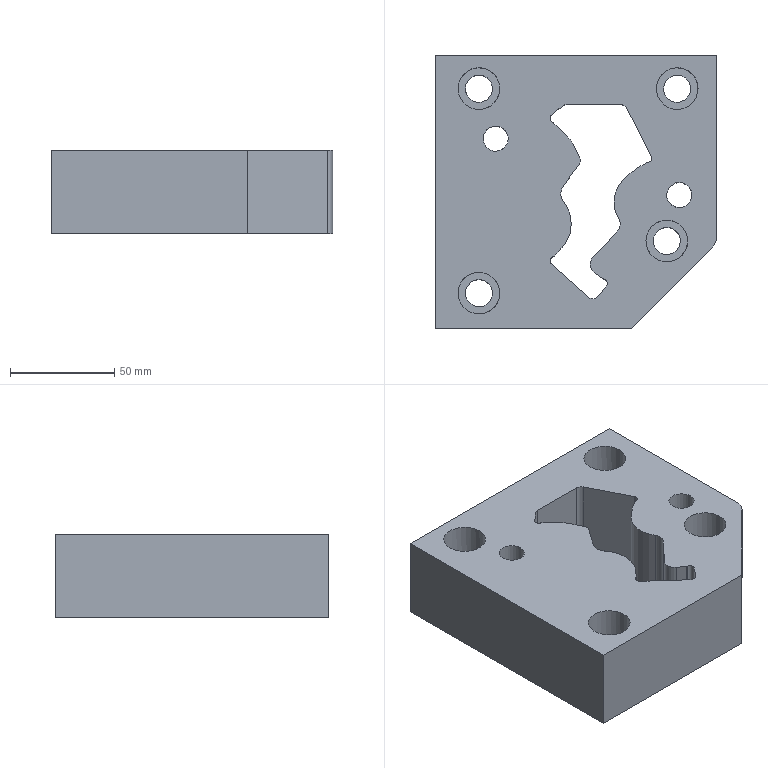Part | STEP file | gslz 2016.10.28-13_id166_x_t | 1 solid | 54 faces | box 135 x 131 x 40 mm | volume 536129 mm3 | cylinder 31 | plane 23 | commonest cylinder face diameters 4 x8 20 x5 6 x4 13 x4 12 x3 10 x2